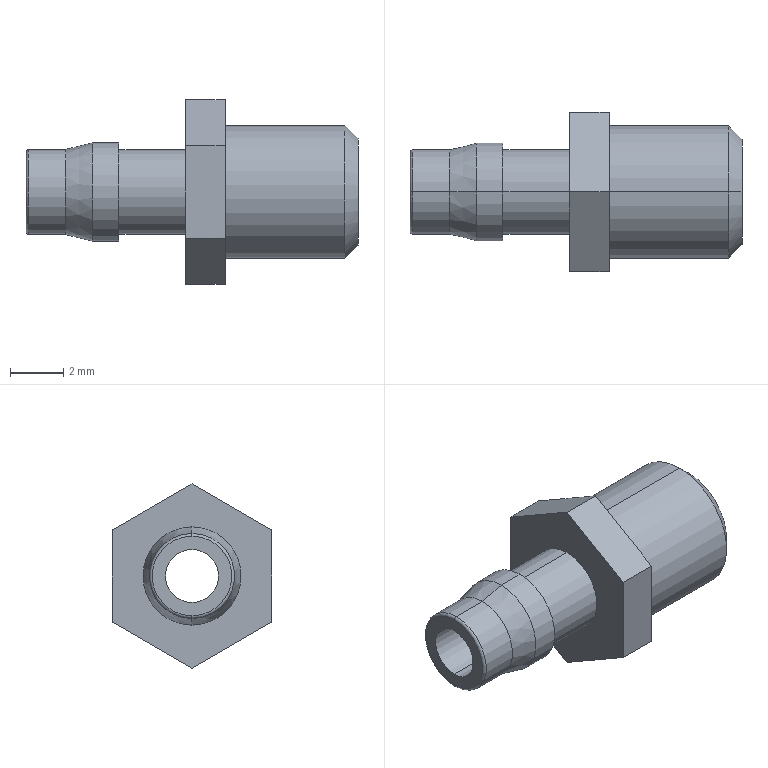Part | SolidWorks | features Chamfer 1, Fillet 1, ICE 1, Revolution 1 | 1 solid | 27 faces | box 12.5 x 6 x 6.928 mm | volume 156.103 mm3 | plane 11 | cylinder 10 | cone 4 | torus 2 | commonest cylinder face diameters 3.2 x4 2 x2 3.7 x2 5 x2
STEP:
#1=CARTESIAN_POINT('',(12.5,0.,-2.));
#2=VERTEX_POINT('',#1);
#3=CARTESIAN_POINT('',(12.5,0.,2.));
#4=VERTEX_POINT('',#3);
#5=CARTESIAN_POINT('',(12.5,0.,0.));
#6=DIRECTION('',(1.,0.,0.));
#7=DIRECTION('',(0.,0.,1.));
#8=AXIS2_PLACEMENT_3D('',#5,#6,#7);
#9=CIRCLE('',#8,2.);
#10=EDGE_CURVE('',#2,#4,#9,.T.);
#11=ORIENTED_EDGE('',*,*,#10,.F.);
#12=CARTESIAN_POINT('',(12.,0.,-2.5));
#13=VERTEX_POINT('',#12);
#14=CARTESIAN_POINT('',(12.,0.,-2.5));
#15=DIRECTION('',(-0.7071,0.,-0.7071));
#16=VECTOR('',#15,1000.);
#17=LINE('',#14,#16);
#18=EDGE_CURVE('',#2,#13,#17,.T.);
#19=ORIENTED_EDGE('',*,*,#18,.T.);
#20=CARTESIAN_POINT('',(12.,0.,2.5));
#21=VERTEX_POINT('',#20);
#22=CARTESIAN_POINT('',(12.,0.,0.));
#23=DIRECTION('',(-1.,0.,0.));
#24=DIRECTION('',(0.,0.,1.));
#25=AXIS2_PLACEMENT_3D('',#22,#23,#24);
#26=CIRCLE('',#25,2.5);
#27=EDGE_CURVE('',#21,#13,#26,.T.);
#28=ORIENTED_EDGE('',*,*,#27,.F.);
#29=CARTESIAN_POINT('',(12.,0.,2.5));
#30=DIRECTION('',(-0.7071,0.,0.7071));
#31=VECTOR('',#30,1000.);
#32=LINE('',#29,#31);
#33=EDGE_CURVE('',#4,#21,#32,.T.);
#34=ORIENTED_EDGE('',*,*,#33,.F.);
#35=EDGE_LOOP('',(#11,#19,#28,#34));
#36=FACE_OUTER_BOUND('',#35,.T.);
#37=CARTESIAN_POINT('',(12.,0.,0.));
#38=DIRECTION('',(-1.,0.,0.));
#39=DIRECTION('',(0.,0.,1.));
#40=AXIS2_PLACEMENT_3D('',#37,#38,#39);
#41=CONICAL_SURFACE('',#40,2.5,0.7854);
#42=ADVANCED_FACE('',(#36),#41,.T.);
#43=CARTESIAN_POINT('',(0.,0.,1.5));
#44=VERTEX_POINT('',#43);
#45=CARTESIAN_POINT('',(0.,0.,-1.5));
#46=VERTEX_POINT('',#45);
#47=CARTESIAN_POINT('',(0.,0.,0.));
#48=DIRECTION('',(-1.,0.,0.));
#49=DIRECTION('',(0.,0.,-1.));
#50=AXIS2_PLACEMENT_3D('',#47,#48,#49);
#51=CIRCLE('',#50,1.5);
#52=EDGE_CURVE('',#44,#46,#51,.T.);
#53=ORIENTED_EDGE('',*,*,#52,.F.);
#54=CARTESIAN_POINT('',(0.1,0.,1.6));
#55=VERTEX_POINT('',#54);
#56=CARTESIAN_POINT('',(0.1,0.,1.5));
#57=DIRECTION('',(0.,1.,0.));
#58=DIRECTION('',(0.,0.,1.));
#59=AXIS2_PLACEMENT_3D('',#56,#57,#58);
#60=CIRCLE('',#59,0.1);
#61=EDGE_CURVE('',#44,#55,#60,.T.);
#62=ORIENTED_EDGE('',*,*,#61,.T.);
#63=CARTESIAN_POINT('',(0.1,0.,-1.6));
#64=VERTEX_POINT('',#63);
#65=CARTESIAN_POINT('',(0.1,0.,0.));
#66=DIRECTION('',(1.,0.,0.));
#67=DIRECTION('',(0.,0.,-1.));
#68=AXIS2_PLACEMENT_3D('',#65,#66,#67);
#69=CIRCLE('',#68,1.6);
#70=EDGE_CURVE('',#64,#55,#69,.T.);
#71=ORIENTED_EDGE('',*,*,#70,.F.);
#72=CARTESIAN_POINT('',(0.1,0.,-1.5));
#73=DIRECTION('',(0.,-1.,0.));
#74=DIRECTION('',(0.,0.,-1.));
#75=AXIS2_PLACEMENT_3D('',#72,#73,#74);
#76=CIRCLE('',#75,0.1);
#77=EDGE_CURVE('',#46,#64,#76,.T.);
#78=ORIENTED_EDGE('',*,*,#77,.F.);
#79=EDGE_LOOP('',(#53,#62,#71,#78));
#80=FACE_OUTER_BOUND('',#79,.T.);
#81=CARTESIAN_POINT('',(0.1,0.,0.));
#82=DIRECTION('',(1.,0.,0.));
#83=DIRECTION('',(0.,0.,-1.));
#84=AXIS2_PLACEMENT_3D('',#81,#82,#83);
#85=TOROIDAL_SURFACE('',#84,1.5,0.1);
#86=ADVANCED_FACE('',(#80),#85,.T.);
#87=CARTESIAN_POINT('',(12.5,0.,-1.));
#88=VERTEX_POINT('',#87);
#89=CARTESIAN_POINT('',(12.5,0.,1.));
#90=VERTEX_POINT('',#89);
#91=CARTESIAN_POINT('',(12.5,0.,0.));
#92=DIRECTION('',(-1.,0.,0.));
#93=DIRECTION('',(0.,0.,1.));
#94=AXIS2_PLACEMENT_3D('',#91,#92,#93);
#95=CIRCLE('',#94,1.);
#96=EDGE_CURVE('',#88,#90,#95,.T.);
#97=ORIENTED_EDGE('',*,*,#96,.F.);
#98=CARTESIAN_POINT('',(0.,0.,-1.));
#99=VERTEX_POINT('',#98);
#100=CARTESIAN_POINT('',(0.,0.,-1.));
#101=DIRECTION('',(-1.,0.,0.));
#102=VECTOR('',#101,1000.);
#103=LINE('',#100,#102);
#104=EDGE_CURVE('',#88,#99,#103,.T.);
#105=ORIENTED_EDGE('',*,*,#104,.T.);
#106=CARTESIAN_POINT('',(0.,0.,1.));
#107=VERTEX_POINT('',#106);
#108=CARTESIAN_POINT('',(0.,0.,0.));
#109=DIRECTION('',(-1.,0.,0.));
#110=DIRECTION('',(0.,0.,1.));
#111=AXIS2_PLACEMENT_3D('',#108,#109,#110);
#112=CIRCLE('',#111,1.);
#113=EDGE_CURVE('',#99,#107,#112,.T.);
#114=ORIENTED_EDGE('',*,*,#113,.T.);
#115=CARTESIAN_POINT('',(0.,0.,1.));
#116=DIRECTION('',(-1.,0.,0.));
#117=VECTOR('',#116,1000.);
#118=LINE('',#115,#117);
#119=EDGE_CURVE('',#90,#107,#118,.T.);
#120=ORIENTED_EDGE('',*,*,#119,.F.);
#121=EDGE_LOOP('',(#97,#105,#114,#120));
#122=FACE_OUTER_BOUND('',#121,.T.);
#123=CARTESIAN_POINT('',(0.,0.,0.));
#124=DIRECTION('',(-1.,0.,0.));
#125=DIRECTION('',(0.,0.,1.));
#126=AXIS2_PLACEMENT_3D('',#123,#124,#125);
#127=CYLINDRICAL_SURFACE('',#126,1.);
#128=ADVANCED_FACE('',(#122),#127,.F.);
#129=ORIENTED_EDGE('',*,*,#27,.T.);
#130=CARTESIAN_POINT('',(7.5,0.,-2.5));
#131=VERTEX_POINT('',#130);
#132=CARTESIAN_POINT('',(0.,0.,-2.5));
#133=DIRECTION('',(-1.,0.,0.));
#134=VECTOR('',#133,1000.);
#135=LINE('',#132,#134);
#136=EDGE_CURVE('',#13,#131,#135,.T.);
#137=ORIENTED_EDGE('',*,*,#136,.T.);
#138=CARTESIAN_POINT('',(7.5,0.,2.5));
#139=VERTEX_POINT('',#138);
#140=CARTESIAN_POINT('',(7.5,0.,0.));
#141=DIRECTION('',(-1.,0.,0.));
#142=DIRECTION('',(0.,0.,1.));
#143=AXIS2_PLACEMENT_3D('',#140,#141,#142);
#144=CIRCLE('',#143,2.5);
#145=EDGE_CURVE('',#139,#131,#144,.T.);
#146=ORIENTED_EDGE('',*,*,#145,.F.);
#147=CARTESIAN_POINT('',(0.,0.,2.5));
#148=DIRECTION('',(-1.,0.,0.));
#149=VECTOR('',#148,1000.);
#150=LINE('',#147,#149);
#151=EDGE_CURVE('',#21,#139,#150,.T.);
#152=ORIENTED_EDGE('',*,*,#151,.F.);
#153=EDGE_LOOP('',(#129,#137,#146,#152));
#154=FACE_OUTER_BOUND('',#153,.T.);
#155=CARTESIAN_POINT('',(0.,0.,0.));
#156=DIRECTION('',(-1.,0.,0.));
#157=DIRECTION('',(0.,0.,1.));
#158=AXIS2_PLACEMENT_3D('',#155,#156,#157);
#159=CYLINDRICAL_SURFACE('',#158,2.5);
#160=ADVANCED_FACE('',(#154),#159,.T.);
#161=CARTESIAN_POINT('',(6.,0.,1.6));
#162=VERTEX_POINT('',#161);
#163=CARTESIAN_POINT('',(6.,0.,-1.6));
#164=VERTEX_POINT('',#163);
#165=CARTESIAN_POINT('',(6.,0.,0.));
#166=DIRECTION('',(-1.,0.,0.));
#167=DIRECTION('',(0.,0.,1.));
#168=AXIS2_PLACEMENT_3D('',#165,#166,#167);
#169=CIRCLE('',#168,1.6);
#170=EDGE_CURVE('',#162,#164,#169,.T.);
#171=ORIENTED_EDGE('',*,*,#170,.T.);
#172=CARTESIAN_POINT('',(3.5,0.,-1.6));
#173=VERTEX_POINT('',#172);
#174=CARTESIAN_POINT('',(0.,0.,-1.6));
#175=DIRECTION('',(-1.,0.,0.));
#176=VECTOR('',#175,1000.);
#177=LINE('',#174,#176);
#178=EDGE_CURVE('',#164,#173,#177,.T.);
#179=ORIENTED_EDGE('',*,*,#178,.T.);
#180=CARTESIAN_POINT('',(3.5,0.,1.6));
#181=VERTEX_POINT('',#180);
#182=CARTESIAN_POINT('',(3.5,0.,0.));
#183=DIRECTION('',(-1.,0.,0.));
#184=DIRECTION('',(0.,0.,1.));
#185=AXIS2_PLACEMENT_3D('',#182,#183,#184);
#186=CIRCLE('',#185,1.6);
#187=EDGE_CURVE('',#181,#173,#186,.T.);
#188=ORIENTED_EDGE('',*,*,#187,.F.);
#189=CARTESIAN_POINT('',(0.,0.,1.6));
#190=DIRECTION('',(-1.,0.,0.));
#191=VECTOR('',#190,1000.);
#192=LINE('',#189,#191);
#193=EDGE_CURVE('',#162,#181,#192,.T.);
#194=ORIENTED_EDGE('',*,*,#193,.F.);
#195=EDGE_LOOP('',(#171,#179,#188,#194));
#196=FACE_OUTER_BOUND('',#195,.T.);
#197=CARTESIAN_POINT('',(0.,0.,0.));
#198=DIRECTION('',(-1.,0.,0.));
#199=DIRECTION('',(0.,0.,1.));
#200=AXIS2_PLACEMENT_3D('',#197,#198,#199);
#201=CYLINDRICAL_SURFACE('',#200,1.6);
#202=ADVANCED_FACE('',(#196),#201,.T.);
#203=CARTESIAN_POINT('',(3.5,0.,1.85));
#204=VERTEX_POINT('',#203);
#205=CARTESIAN_POINT('',(3.5,0.,-1.85));
#206=VERTEX_POINT('',#205);
#207=CARTESIAN_POINT('',(3.5,0.,0.));
#208=DIRECTION('',(-1.,0.,0.));
#209=DIRECTION('',(0.,0.,1.));
#210=AXIS2_PLACEMENT_3D('',#207,#208,#209);
#211=CIRCLE('',#210,1.85);
#212=EDGE_CURVE('',#204,#206,#211,.T.);
#213=ORIENTED_EDGE('',*,*,#212,.T.);
#214=CARTESIAN_POINT('',(2.5,0.,-1.85));
#215=VERTEX_POINT('',#214);
#216=CARTESIAN_POINT('',(0.,0.,-1.85));
#217=DIRECTION('',(-1.,0.,0.));
#218=VECTOR('',#217,1000.);
#219=LINE('',#216,#218);
#220=EDGE_CURVE('',#206,#215,#219,.T.);
#221=ORIENTED_EDGE('',*,*,#220,.T.);
#222=CARTESIAN_POINT('',(2.5,0.,1.85));
#223=VERTEX_POINT('',#222);
#224=CARTESIAN_POINT('',(2.5,0.,0.));
#225=DIRECTION('',(-1.,0.,0.));
#226=DIRECTION('',(0.,0.,1.));
#227=AXIS2_PLACEMENT_3D('',#224,#225,#226);
#228=CIRCLE('',#227,1.85);
#229=EDGE_CURVE('',#223,#215,#228,.T.);
#230=ORIENTED_EDGE('',*,*,#229,.F.);
#231=CARTESIAN_POINT('',(0.,0.,1.85));
#232=DIRECTION('',(-1.,0.,0.));
#233=VECTOR('',#232,1000.);
#234=LINE('',#231,#233);
#235=EDGE_CURVE('',#204,#223,#234,.T.);
#236=ORIENTED_EDGE('',*,*,#235,.F.);
#237=EDGE_LOOP('',(#213,#221,#230,#236));
#238=FACE_OUTER_BOUND('',#237,.T.);
#239=CARTESIAN_POINT('',(0.,0.,0.));
#240=DIRECTION('',(-1.,0.,0.));
#241=DIRECTION('',(0.,0.,1.));
#242=AXIS2_PLACEMENT_3D('',#239,#240,#241);
#243=CYLINDRICAL_SURFACE('',#242,1.85);
#244=ADVANCED_FACE('',(#238),#243,.T.);
#245=CARTESIAN_POINT('',(1.5,0.,1.6));
#246=VERTEX_POINT('',#245);
#247=CARTESIAN_POINT('',(1.5,0.,-1.6));
#248=VERTEX_POINT('',#247);
#249=CARTESIAN_POINT('',(1.5,0.,0.));
#250=DIRECTION('',(-1.,0.,0.));
#251=DIRECTION('',(0.,0.,1.));
#252=AXIS2_PLACEMENT_3D('',#249,#250,#251);
#253=CIRCLE('',#252,1.6);
#254=EDGE_CURVE('',#246,#248,#253,.T.);
#255=ORIENTED_EDGE('',*,*,#254,.F.);
#256=CARTESIAN_POINT('',(2.5,0.,1.85));
#257=DIRECTION('',(0.9701,0.,0.2425));
#258=VECTOR('',#257,1000.);
#259=LINE('',#256,#258);
#260=EDGE_CURVE('',#246,#223,#259,.T.);
#261=ORIENTED_EDGE('',*,*,#260,.T.);
#262=ORIENTED_EDGE('',*,*,#229,.T.);
#263=CARTESIAN_POINT('',(2.5,0.,-1.85));
#264=DIRECTION('',(0.9701,0.,-0.2425));
#265=VECTOR('',#264,1000.);
#266=LINE('',#263,#265);
#267=EDGE_CURVE('',#248,#215,#266,.T.);
#268=ORIENTED_EDGE('',*,*,#267,.F.);
#269=EDGE_LOOP('',(#255,#261,#262,#268));
#270=FACE_OUTER_BOUND('',#269,.T.);
#271=CARTESIAN_POINT('',(2.5,0.,0.));
#272=DIRECTION('',(1.,0.,0.));
#273=DIRECTION('',(0.,0.,-1.));
#274=AXIS2_PLACEMENT_3D('',#271,#272,#273);
#275=CONICAL_SURFACE('',#274,1.85,0.245);
#276=ADVANCED_FACE('',(#270),#275,.T.);
#277=ORIENTED_EDGE('',*,*,#254,.T.);
#278=CARTESIAN_POINT('',(0.,0.,-1.6));
#279=DIRECTION('',(-1.,0.,0.));
#280=VECTOR('',#279,1000.);
#281=LINE('',#278,#280);
#282=EDGE_CURVE('',#248,#64,#281,.T.);
#283=ORIENTED_EDGE('',*,*,#282,.T.);
#284=ORIENTED_EDGE('',*,*,#70,.T.);
#285=CARTESIAN_POINT('',(0.,0.,1.6));
#286=DIRECTION('',(-1.,0.,0.));
#287=VECTOR('',#286,1000.);
#288=LINE('',#285,#287);
#289=EDGE_CURVE('',#246,#55,#288,.T.);
#290=ORIENTED_EDGE('',*,*,#289,.F.);
#291=EDGE_LOOP('',(#277,#283,#284,#290));
#292=FACE_OUTER_BOUND('',#291,.T.);
#293=CARTESIAN_POINT('',(0.,0.,0.));
#294=DIRECTION('',(-1.,0.,0.));
#295=DIRECTION('',(0.,0.,1.));
#296=AXIS2_PLACEMENT_3D('',#293,#294,#295);
#297=CYLINDRICAL_SURFACE('',#296,1.6);
#298=ADVANCED_FACE('',(#292),#297,.T.);
#299=ORIENTED_EDGE('',*,*,#170,.F.);
#300=CARTESIAN_POINT('',(6.,0.,0.));
#301=DIRECTION('',(-1.,0.,0.));
#302=DIRECTION('',(0.,0.,1.));
#303=AXIS2_PLACEMENT_3D('',#300,#301,#302);
#304=CIRCLE('',#303,1.6);
#305=EDGE_CURVE('',#164,#162,#304,.T.);
#306=ORIENTED_EDGE('',*,*,#305,.F.);
#307=EDGE_LOOP('',(#299,#306));
#308=FACE_BOUND('',#307,.T.);
#309=CARTESIAN_POINT('',(6.,-3.,1.732));
#310=VERTEX_POINT('',#309);
#311=CARTESIAN_POINT('',(6.,-3.,-1.732));
#312=VERTEX_POINT('',#311);
#313=CARTESIAN_POINT('',(6.,-3.,0.));
#314=DIRECTION('',(0.,0.,-1.));
#315=VECTOR('',#314,1000.);
#316=LINE('',#313,#315);
#317=EDGE_CURVE('',#310,#312,#316,.T.);
#318=ORIENTED_EDGE('',*,*,#317,.F.);
#319=CARTESIAN_POINT('',(6.,0.,3.464));
#320=VERTEX_POINT('',#319);
#321=CARTESIAN_POINT('',(6.,-0.3,3.291));
#322=DIRECTION('',(0.,-0.866,-0.5));
#323=VECTOR('',#322,1000.);
#324=LINE('',#321,#323);
#325=EDGE_CURVE('',#320,#310,#324,.T.);
#326=ORIENTED_EDGE('',*,*,#325,.F.);
#327=CARTESIAN_POINT('',(6.,3.,1.732));
#328=VERTEX_POINT('',#327);
#329=CARTESIAN_POINT('',(6.,2.7,1.905));
#330=DIRECTION('',(0.,-0.866,0.5));
#331=VECTOR('',#330,1000.);
#332=LINE('',#329,#331);
#333=EDGE_CURVE('',#328,#320,#332,.T.);
#334=ORIENTED_EDGE('',*,*,#333,.F.);
#335=CARTESIAN_POINT('',(6.,3.,-1.732));
#336=VERTEX_POINT('',#335);
#337=CARTESIAN_POINT('',(6.,3.,0.));
#338=DIRECTION('',(0.,0.,1.));
#339=VECTOR('',#338,1000.);
#340=LINE('',#337,#339);
#341=EDGE_CURVE('',#336,#328,#340,.T.);
#342=ORIENTED_EDGE('',*,*,#341,.F.);
#343=CARTESIAN_POINT('',(6.,0.,-3.464));
#344=VERTEX_POINT('',#343);
#345=CARTESIAN_POINT('',(6.,2.7,-1.905));
#346=DIRECTION('',(0.,0.866,0.5));
#347=VECTOR('',#346,1000.);
#348=LINE('',#345,#347);
#349=EDGE_CURVE('',#344,#336,#348,.T.);
#350=ORIENTED_EDGE('',*,*,#349,.F.);
#351=CARTESIAN_POINT('',(6.,-0.3,-3.291));
#352=DIRECTION('',(0.,0.866,-0.5));
#353=VECTOR('',#352,1000.);
#354=LINE('',#351,#353);
#355=EDGE_CURVE('',#312,#344,#354,.T.);
#356=ORIENTED_EDGE('',*,*,#355,.F.);
#357=EDGE_LOOP('',(#318,#326,#334,#342,#350,#356));
#358=FACE_OUTER_BOUND('',#357,.T.);
#359=CARTESIAN_POINT('',(6.,1.6,0.));
#360=DIRECTION('',(1.,0.,0.));
#361=DIRECTION('',(0.,0.,-1.));
#362=AXIS2_PLACEMENT_3D('',#359,#360,#361);
#363=PLANE('',#362);
#364=ADVANCED_FACE('',(#308,#358),#363,.F.);
#365=ORIENTED_EDGE('',*,*,#145,.T.);
#366=CARTESIAN_POINT('',(7.5,0.,0.));
#367=DIRECTION('',(-1.,0.,0.));
#368=DIRECTION('',(0.,0.,1.));
#369=AXIS2_PLACEMENT_3D('',#366,#367,#368);
#370=CIRCLE('',#369,2.5);
#371=EDGE_CURVE('',#131,#139,#370,.T.);
#372=ORIENTED_EDGE('',*,*,#371,.T.);
#373=EDGE_LOOP('',(#365,#372));
#374=FACE_BOUND('',#373,.T.);
#375=CARTESIAN_POINT('',(7.5,-3.,1.732));
#376=VERTEX_POINT('',#375);
#377=CARTESIAN_POINT('',(7.5,-3.,-1.732));
#378=VERTEX_POINT('',#377);
#379=CARTESIAN_POINT('',(7.5,-3.,1.732));
#380=DIRECTION('',(0.,0.,-1.));
#381=VECTOR('',#380,1000.);
#382=LINE('',#379,#381);
#383=EDGE_CURVE('',#376,#378,#382,.T.);
#384=ORIENTED_EDGE('',*,*,#383,.T.);
#385=CARTESIAN_POINT('',(7.5,0.,-3.464));
#386=VERTEX_POINT('',#385);
#387=CARTESIAN_POINT('',(7.5,-3.,-1.732));
#388=DIRECTION('',(0.,0.866,-0.5));
#389=VECTOR('',#388,1000.);
#390=LINE('',#387,#389);
#391=EDGE_CURVE('',#378,#386,#390,.T.);
#392=ORIENTED_EDGE('',*,*,#391,.T.);
#393=CARTESIAN_POINT('',(7.5,3.,-1.732));
#394=VERTEX_POINT('',#393);
#395=CARTESIAN_POINT('',(7.5,0.,-3.464));
#396=DIRECTION('',(0.,0.866,0.5));
#397=VECTOR('',#396,1000.);
#398=LINE('',#395,#397);
#399=EDGE_CURVE('',#386,#394,#398,.T.);
#400=ORIENTED_EDGE('',*,*,#399,.T.);
#401=CARTESIAN_POINT('',(7.5,3.,1.732));
#402=VERTEX_POINT('',#401);
#403=CARTESIAN_POINT('',(7.5,3.,-1.732));
#404=DIRECTION('',(0.,0.,1.));
#405=VECTOR('',#404,1000.);
#406=LINE('',#403,#405);
#407=EDGE_CURVE('',#394,#402,#406,.T.);
#408=ORIENTED_EDGE('',*,*,#407,.T.);
#409=CARTESIAN_POINT('',(7.5,0.,3.464));
#410=VERTEX_POINT('',#409);
#411=CARTESIAN_POINT('',(7.5,3.,1.732));
#412=DIRECTION('',(0.,-0.866,0.5));
#413=VECTOR('',#412,1000.);
#414=LINE('',#411,#413);
#415=EDGE_CURVE('',#402,#410,#414,.T.);
#416=ORIENTED_EDGE('',*,*,#415,.T.);
#417=CARTESIAN_POINT('',(7.5,0.,3.464));
#418=DIRECTION('',(0.,-0.866,-0.5));
#419=VECTOR('',#418,1000.);
#420=LINE('',#417,#419);
#421=EDGE_CURVE('',#410,#376,#420,.T.);
#422=ORIENTED_EDGE('',*,*,#421,.T.);
#423=EDGE_LOOP('',(#384,#392,#400,#408,#416,#422));
#424=FACE_OUTER_BOUND('',#423,.T.);
#425=CARTESIAN_POINT('',(7.5,4.5,0.));
#426=DIRECTION('',(-1.,0.,0.));
#427=DIRECTION('',(0.,0.,1.));
#428=AXIS2_PLACEMENT_3D('',#425,#426,#427);
#429=PLANE('',#428);
#430=ADVANCED_FACE('',(#374,#424),#429,.F.);
#431=CARTESIAN_POINT('',(0.,0.,0.));
#432=DIRECTION('',(-1.,0.,0.));
#433=DIRECTION('',(0.,0.,-1.));
#434=AXIS2_PLACEMENT_3D('',#431,#432,#433);
#435=CIRCLE('',#434,1.5);
#436=EDGE_CURVE('',#46,#44,#435,.T.);
#437=ORIENTED_EDGE('',*,*,#436,.T.);
#438=ORIENTED_EDGE('',*,*,#52,.T.);
#439=EDGE_LOOP('',(#437,#438));
#440=FACE_OUTER_BOUND('',#439,.T.);
#441=CARTESIAN_POINT('',(0.,0.,0.));
#442=DIRECTION('',(-1.,0.,0.));
#443=DIRECTION('',(0.,0.,1.));
#444=AXIS2_PLACEMENT_3D('',#441,#442,#443);
#445=CIRCLE('',#444,1.);
#446=EDGE_CURVE('',#107,#99,#445,.T.);
#447=ORIENTED_EDGE('',*,*,#446,.F.);
#448=ORIENTED_EDGE('',*,*,#113,.F.);
#449=EDGE_LOOP('',(#447,#448));
#450=FACE_BOUND('',#449,.T.);
#451=CARTESIAN_POINT('',(0.,1.,0.));
#452=DIRECTION('',(1.,0.,0.));
#453=DIRECTION('',(0.,0.,-1.));
#454=AXIS2_PLACEMENT_3D('',#451,#452,#453);
#455=PLANE('',#454);
#456=ADVANCED_FACE('',(#440,#450),#455,.F.);
#457=ORIENTED_EDGE('',*,*,#282,.F.);
#458=CARTESIAN_POINT('',(1.5,0.,0.));
#459=DIRECTION('',(-1.,0.,0.));
#460=DIRECTION('',(0.,0.,1.));
#461=AXIS2_PLACEMENT_3D('',#458,#459,#460);
#462=CIRCLE('',#461,1.6);
#463=EDGE_CURVE('',#248,#246,#462,.T.);
#464=ORIENTED_EDGE('',*,*,#463,.T.);
#465=ORIENTED_EDGE('',*,*,#289,.T.);
#466=CARTESIAN_POINT('',(0.1,0.,0.));
#467=DIRECTION('',(1.,0.,0.));
#468=DIRECTION('',(0.,0.,-1.));
#469=AXIS2_PLACEMENT_3D('',#466,#467,#468);
#470=CIRCLE('',#469,1.6);
#471=EDGE_CURVE('',#55,#64,#470,.T.);
#472=ORIENTED_EDGE('',*,*,#471,.T.);
#473=EDGE_LOOP('',(#457,#464,#465,#472));
#474=FACE_OUTER_BOUND('',#473,.T.);
#475=CARTESIAN_POINT('',(0.,0.,0.));
#476=DIRECTION('',(-1.,0.,0.));
#477=DIRECTION('',(0.,0.,1.));
#478=AXIS2_PLACEMENT_3D('',#475,#476,#477);
#479=CYLINDRICAL_SURFACE('',#478,1.6);
#480=ADVANCED_FACE('',(#474),#479,.T.);
#481=ORIENTED_EDGE('',*,*,#260,.F.);
#482=ORIENTED_EDGE('',*,*,#463,.F.);
#483=ORIENTED_EDGE('',*,*,#267,.T.);
#484=CARTESIAN_POINT('',(2.5,0.,0.));
#485=DIRECTION('',(-1.,0.,0.));
#486=DIRECTION('',(0.,0.,1.));
#487=AXIS2_PLACEMENT_3D('',#484,#485,#486);
#488=CIRCLE('',#487,1.85);
#489=EDGE_CURVE('',#215,#223,#488,.T.);
#490=ORIENTED_EDGE('',*,*,#489,.T.);
#491=EDGE_LOOP('',(#481,#482,#483,#490));
#492=FACE_OUTER_BOUND('',#491,.T.);
#493=CARTESIAN_POINT('',(2.5,0.,0.));
#494=DIRECTION('',(1.,0.,0.));
#495=DIRECTION('',(0.,0.,-1.));
#496=AXIS2_PLACEMENT_3D('',#493,#494,#495);
#497=CONICAL_SURFACE('',#496,1.85,0.245);
#498=ADVANCED_FACE('',(#492),#497,.T.);
#499=ORIENTED_EDGE('',*,*,#220,.F.);
#500=CARTESIAN_POINT('',(3.5,0.,0.));
#501=DIRECTION('',(-1.,0.,0.));
#502=DIRECTION('',(0.,0.,1.));
#503=AXIS2_PLACEMENT_3D('',#500,#501,#502);
#504=CIRCLE('',#503,1.85);
#505=EDGE_CURVE('',#206,#204,#504,.T.);
#506=ORIENTED_EDGE('',*,*,#505,.T.);
#507=ORIENTED_EDGE('',*,*,#235,.T.);
#508=ORIENTED_EDGE('',*,*,#489,.F.);
#509=EDGE_LOOP('',(#499,#506,#507,#508));
#510=FACE_OUTER_BOUND('',#509,.T.);
#511=CARTESIAN_POINT('',(0.,0.,0.));
#512=DIRECTION('',(-1.,0.,0.));
#513=DIRECTION('',(0.,0.,1.));
#514=AXIS2_PLACEMENT_3D('',#511,#512,#513);
#515=CYLINDRICAL_SURFACE('',#514,1.85);
#516=ADVANCED_FACE('',(#510),#515,.T.);
#517=ORIENTED_EDGE('',*,*,#212,.F.);
#518=ORIENTED_EDGE('',*,*,#505,.F.);
#519=EDGE_LOOP('',(#517,#518));
#520=FACE_OUTER_BOUND('',#519,.T.);
#521=ORIENTED_EDGE('',*,*,#187,.T.);
#522=CARTESIAN_POINT('',(3.5,0.,0.));
#523=DIRECTION('',(-1.,0.,0.));
#524=DIRECTION('',(0.,0.,1.));
#525=AXIS2_PLACEMENT_3D('',#522,#523,#524);
#526=CIRCLE('',#525,1.6);
#527=EDGE_CURVE('',#173,#181,#526,.T.);
#528=ORIENTED_EDGE('',*,*,#527,.T.);
#529=EDGE_LOOP('',(#521,#528));
#530=FACE_BOUND('',#529,.T.);
#531=CARTESIAN_POINT('',(3.5,1.85,0.));
#532=DIRECTION('',(-1.,0.,0.));
#533=DIRECTION('',(0.,0.,1.));
#534=AXIS2_PLACEMENT_3D('',#531,#532,#533);
#535=PLANE('',#534);
#536=ADVANCED_FACE('',(#520,#530),#535,.F.);
#537=ORIENTED_EDGE('',*,*,#178,.F.);
#538=ORIENTED_EDGE('',*,*,#305,.T.);
#539=ORIENTED_EDGE('',*,*,#193,.T.);
#540=ORIENTED_EDGE('',*,*,#527,.F.);
#541=EDGE_LOOP('',(#537,#538,#539,#540));
#542=FACE_OUTER_BOUND('',#541,.T.);
#543=CARTESIAN_POINT('',(0.,0.,0.));
#544=DIRECTION('',(-1.,0.,0.));
#545=DIRECTION('',(0.,0.,1.));
#546=AXIS2_PLACEMENT_3D('',#543,#544,#545);
#547=CYLINDRICAL_SURFACE('',#546,1.6);
#548=ADVANCED_FACE('',(#542),#547,.T.);
#549=ORIENTED_EDGE('',*,*,#136,.F.);
#550=CARTESIAN_POINT('',(12.,0.,0.));
#551=DIRECTION('',(-1.,0.,0.));
#552=DIRECTION('',(0.,0.,1.));
#553=AXIS2_PLACEMENT_3D('',#550,#551,#552);
#554=CIRCLE('',#553,2.5);
#555=EDGE_CURVE('',#13,#21,#554,.T.);
#556=ORIENTED_EDGE('',*,*,#555,.T.);
#557=ORIENTED_EDGE('',*,*,#151,.T.);
#558=ORIENTED_EDGE('',*,*,#371,.F.);
#559=EDGE_LOOP('',(#549,#556,#557,#558));
#560=FACE_OUTER_BOUND('',#559,.T.);
#561=CARTESIAN_POINT('',(0.,0.,0.));
#562=DIRECTION('',(-1.,0.,0.));
#563=DIRECTION('',(0.,0.,1.));
#564=AXIS2_PLACEMENT_3D('',#561,#562,#563);
#565=CYLINDRICAL_SURFACE('',#564,2.5);
#566=ADVANCED_FACE('',(#560),#565,.T.);
#567=CARTESIAN_POINT('',(12.5,0.,0.));
#568=DIRECTION('',(1.,0.,0.));
#569=DIRECTION('',(0.,0.,1.));
#570=AXIS2_PLACEMENT_3D('',#567,#568,#569);
#571=CIRCLE('',#570,2.);
#572=EDGE_CURVE('',#4,#2,#571,.T.);
#573=ORIENTED_EDGE('',*,*,#572,.T.);
#574=ORIENTED_EDGE('',*,*,#10,.T.);
#575=EDGE_LOOP('',(#573,#574));
#576=FACE_OUTER_BOUND('',#575,.T.);
#577=CARTESIAN_POINT('',(12.5,0.,0.));
#578=DIRECTION('',(-1.,0.,0.));
#579=DIRECTION('',(0.,0.,1.));
#580=AXIS2_PLACEMENT_3D('',#577,#578,#579);
#581=CIRCLE('',#580,1.);
#582=EDGE_CURVE('',#90,#88,#581,.T.);
#583=ORIENTED_EDGE('',*,*,#582,.T.);
#584=ORIENTED_EDGE('',*,*,#96,.T.);
#585=EDGE_LOOP('',(#583,#584));
#586=FACE_BOUND('',#585,.T.);
#587=CARTESIAN_POINT('',(12.5,2.5,0.));
#588=DIRECTION('',(-1.,0.,0.));
#589=DIRECTION('',(0.,0.,1.));
#590=AXIS2_PLACEMENT_3D('',#587,#588,#589);
#591=PLANE('',#590);
#592=ADVANCED_FACE('',(#576,#586),#591,.F.);
#593=ORIENTED_EDGE('',*,*,#104,.F.);
#594=ORIENTED_EDGE('',*,*,#582,.F.);
#595=ORIENTED_EDGE('',*,*,#119,.T.);
#596=ORIENTED_EDGE('',*,*,#446,.T.);
#597=EDGE_LOOP('',(#593,#594,#595,#596));
#598=FACE_OUTER_BOUND('',#597,.T.);
#599=CARTESIAN_POINT('',(0.,0.,0.));
#600=DIRECTION('',(-1.,0.,0.));
#601=DIRECTION('',(0.,0.,1.));
#602=AXIS2_PLACEMENT_3D('',#599,#600,#601);
#603=CYLINDRICAL_SURFACE('',#602,1.);
#604=ADVANCED_FACE('',(#598),#603,.F.);
#605=ORIENTED_EDGE('',*,*,#317,.T.);
#606=CARTESIAN_POINT('',(-2.5,-3.,-1.732));
#607=DIRECTION('',(1.,0.,0.));
#608=VECTOR('',#607,1000.);
#609=LINE('',#606,#608);
#610=EDGE_CURVE('',#312,#378,#609,.T.);
#611=ORIENTED_EDGE('',*,*,#610,.T.);
#612=ORIENTED_EDGE('',*,*,#383,.F.);
#613=CARTESIAN_POINT('',(-2.5,-3.,1.732));
#614=DIRECTION('',(1.,0.,0.));
#615=VECTOR('',#614,1000.);
#616=LINE('',#613,#615);
#617=EDGE_CURVE('',#310,#376,#616,.T.);
#618=ORIENTED_EDGE('',*,*,#617,.F.);
#619=EDGE_LOOP('',(#605,#611,#612,#618));
#620=FACE_OUTER_BOUND('',#619,.T.);
#621=CARTESIAN_POINT('',(-2.5,-3.,1.732));
#622=DIRECTION('',(0.,-1.,0.));
#623=DIRECTION('',(0.,0.,-1.));
#624=AXIS2_PLACEMENT_3D('',#621,#622,#623);
#625=PLANE('',#624);
#626=ADVANCED_FACE('',(#620),#625,.T.);
#627=ORIENTED_EDGE('',*,*,#325,.T.);
#628=ORIENTED_EDGE('',*,*,#617,.T.);
#629=ORIENTED_EDGE('',*,*,#421,.F.);
#630=CARTESIAN_POINT('',(-2.5,0.,3.464));
#631=DIRECTION('',(1.,0.,0.));
#632=VECTOR('',#631,1000.);
#633=LINE('',#630,#632);
#634=EDGE_CURVE('',#320,#410,#633,.T.);
#635=ORIENTED_EDGE('',*,*,#634,.F.);
#636=EDGE_LOOP('',(#627,#628,#629,#635));
#637=FACE_OUTER_BOUND('',#636,.T.);
#638=CARTESIAN_POINT('',(-2.5,0.,3.464));
#639=DIRECTION('',(0.,-0.5,0.866));
#640=DIRECTION('',(0.,-0.866,-0.5));
#641=AXIS2_PLACEMENT_3D('',#638,#639,#640);
#642=PLANE('',#641);
#643=ADVANCED_FACE('',(#637),#642,.T.);
#644=ORIENTED_EDGE('',*,*,#333,.T.);
#645=ORIENTED_EDGE('',*,*,#634,.T.);
#646=ORIENTED_EDGE('',*,*,#415,.F.);
#647=CARTESIAN_POINT('',(-2.5,3.,1.732));
#648=DIRECTION('',(1.,0.,0.));
#649=VECTOR('',#648,1000.);
#650=LINE('',#647,#649);
#651=EDGE_CURVE('',#328,#402,#650,.T.);
#652=ORIENTED_EDGE('',*,*,#651,.F.);
#653=EDGE_LOOP('',(#644,#645,#646,#652));
#654=FACE_OUTER_BOUND('',#653,.T.);
#655=CARTESIAN_POINT('',(-2.5,3.,1.732));
#656=DIRECTION('',(0.,0.5,0.866));
#657=DIRECTION('',(0.,-0.866,0.5));
#658=AXIS2_PLACEMENT_3D('',#655,#656,#657);
#659=PLANE('',#658);
#660=ADVANCED_FACE('',(#654),#659,.T.);
#661=ORIENTED_EDGE('',*,*,#341,.T.);
#662=ORIENTED_EDGE('',*,*,#651,.T.);
#663=ORIENTED_EDGE('',*,*,#407,.F.);
#664=CARTESIAN_POINT('',(-2.5,3.,-1.732));
#665=DIRECTION('',(1.,0.,0.));
#666=VECTOR('',#665,1000.);
#667=LINE('',#664,#666);
#668=EDGE_CURVE('',#336,#394,#667,.T.);
#669=ORIENTED_EDGE('',*,*,#668,.F.);
#670=EDGE_LOOP('',(#661,#662,#663,#669));
#671=FACE_OUTER_BOUND('',#670,.T.);
#672=CARTESIAN_POINT('',(-2.5,3.,-1.732));
#673=DIRECTION('',(0.,1.,0.));
#674=DIRECTION('',(0.,0.,1.));
#675=AXIS2_PLACEMENT_3D('',#672,#673,#674);
#676=PLANE('',#675);
#677=ADVANCED_FACE('',(#671),#676,.T.);
#678=ORIENTED_EDGE('',*,*,#349,.T.);
#679=ORIENTED_EDGE('',*,*,#668,.T.);
#680=ORIENTED_EDGE('',*,*,#399,.F.);
#681=CARTESIAN_POINT('',(-2.5,0.,-3.464));
#682=DIRECTION('',(1.,0.,0.));
#683=VECTOR('',#682,1000.);
#684=LINE('',#681,#683);
#685=EDGE_CURVE('',#344,#386,#684,.T.);
#686=ORIENTED_EDGE('',*,*,#685,.F.);
#687=EDGE_LOOP('',(#678,#679,#680,#686));
#688=FACE_OUTER_BOUND('',#687,.T.);
#689=CARTESIAN_POINT('',(-2.5,0.,-3.464));
#690=DIRECTION('',(0.,0.5,-0.866));
#691=DIRECTION('',(0.,0.866,0.5));
#692=AXIS2_PLACEMENT_3D('',#689,#690,#691);
#693=PLANE('',#692);
#694=ADVANCED_FACE('',(#688),#693,.T.);
#695=ORIENTED_EDGE('',*,*,#355,.T.);
#696=ORIENTED_EDGE('',*,*,#685,.T.);
#697=ORIENTED_EDGE('',*,*,#391,.F.);
#698=ORIENTED_EDGE('',*,*,#610,.F.);
#699=EDGE_LOOP('',(#695,#696,#697,#698));
#700=FACE_OUTER_BOUND('',#699,.T.);
#701=CARTESIAN_POINT('',(-2.5,-3.,-1.732));
#702=DIRECTION('',(0.,-0.5,-0.866));
#703=DIRECTION('',(0.,0.866,-0.5));
#704=AXIS2_PLACEMENT_3D('',#701,#702,#703);
#705=PLANE('',#704);
#706=ADVANCED_FACE('',(#700),#705,.T.);
#707=ORIENTED_EDGE('',*,*,#61,.F.);
#708=ORIENTED_EDGE('',*,*,#436,.F.);
#709=ORIENTED_EDGE('',*,*,#77,.T.);
#710=ORIENTED_EDGE('',*,*,#471,.F.);
#711=EDGE_LOOP('',(#707,#708,#709,#710));
#712=FACE_OUTER_BOUND('',#711,.T.);
#713=CARTESIAN_POINT('',(0.1,0.,0.));
#714=DIRECTION('',(1.,0.,0.));
#715=DIRECTION('',(0.,0.,-1.));
#716=AXIS2_PLACEMENT_3D('',#713,#714,#715);
#717=TOROIDAL_SURFACE('',#716,1.5,0.1);
#718=ADVANCED_FACE('',(#712),#717,.T.);
#719=ORIENTED_EDGE('',*,*,#18,.F.);
#720=ORIENTED_EDGE('',*,*,#572,.F.);
#721=ORIENTED_EDGE('',*,*,#33,.T.);
#722=ORIENTED_EDGE('',*,*,#555,.F.);
#723=EDGE_LOOP('',(#719,#720,#721,#722));
#724=FACE_OUTER_BOUND('',#723,.T.);
#725=CARTESIAN_POINT('',(12.,0.,0.));
#726=DIRECTION('',(-1.,0.,0.));
#727=DIRECTION('',(0.,0.,1.));
#728=AXIS2_PLACEMENT_3D('',#725,#726,#727);
#729=CONICAL_SURFACE('',#728,2.5,0.7854);
#730=ADVANCED_FACE('',(#724),#729,.T.);
#731=CLOSED_SHELL('',(#42,#86,#128,#160,#202,#244,#276,#298,#364,#430,#456,#480,#498,#516,#536,#548,#566,#592,#604,#626,#643,#660,#677,#694,#706,#718,#730));
#732=MANIFOLD_SOLID_BREP('',#731);
#733=CARTESIAN_POINT('',(0.,0.,0.));
#734=DIRECTION('',(0.,0.,1.));
#735=DIRECTION('',(1.,0.,0.));
#736=AXIS2_PLACEMENT_3D('',#733,#734,#735);
#737=(LENGTH_UNIT()NAMED_UNIT(*)SI_UNIT(.MILLI.,.METRE.));
#738=UNCERTAINTY_MEASURE_WITH_UNIT(LENGTH_MEASURE(0.00001),#737,'','');
#739=(NAMED_UNIT(*)PLANE_ANGLE_UNIT()SI_UNIT($,.RADIAN.));
#740=(NAMED_UNIT(*)SI_UNIT($,.STERADIAN.)SOLID_ANGLE_UNIT());
#741=(GEOMETRIC_REPRESENTATION_CONTEXT(3)GLOBAL_UNCERTAINTY_ASSIGNED_CONTEXT((#738))GLOBAL_UNIT_ASSIGNED_CONTEXT((#737,#739,#740))REPRESENTATION_CONTEXT('',''));
#742=ADVANCED_BREP_SHAPE_REPRESENTATION('',(#732,#736),#741);